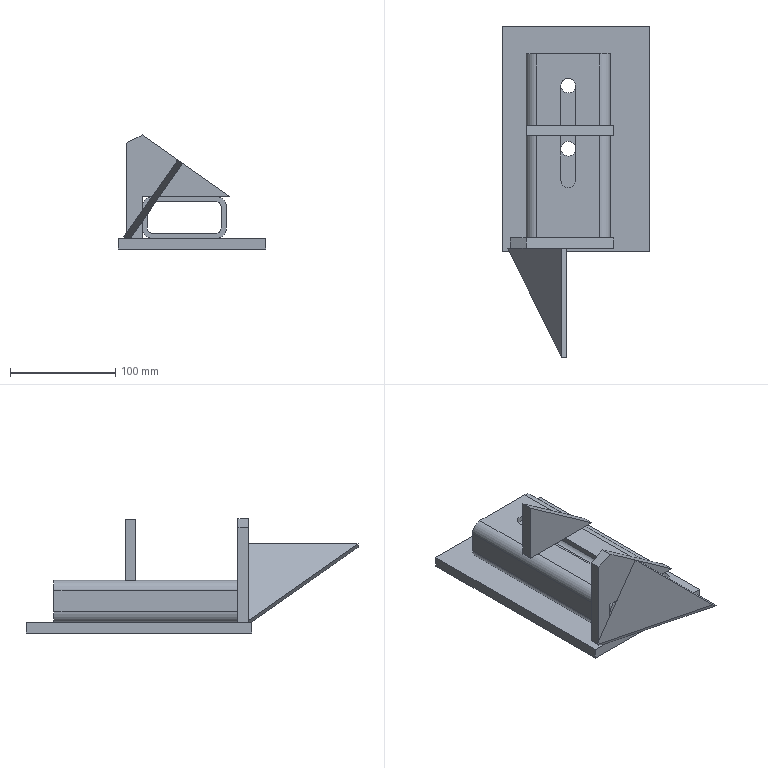Part | STEP file | rectangular upper-left upper why latest oblique change-
-2025.12.03 | 5 solids | 52 faces | box 140.025 x 315.696 x 108.411 mm | volume 564954 mm3 | plane 38 | cylinder 14 | commonest cylinder face diameters 14 x6 10 x4 20 x4